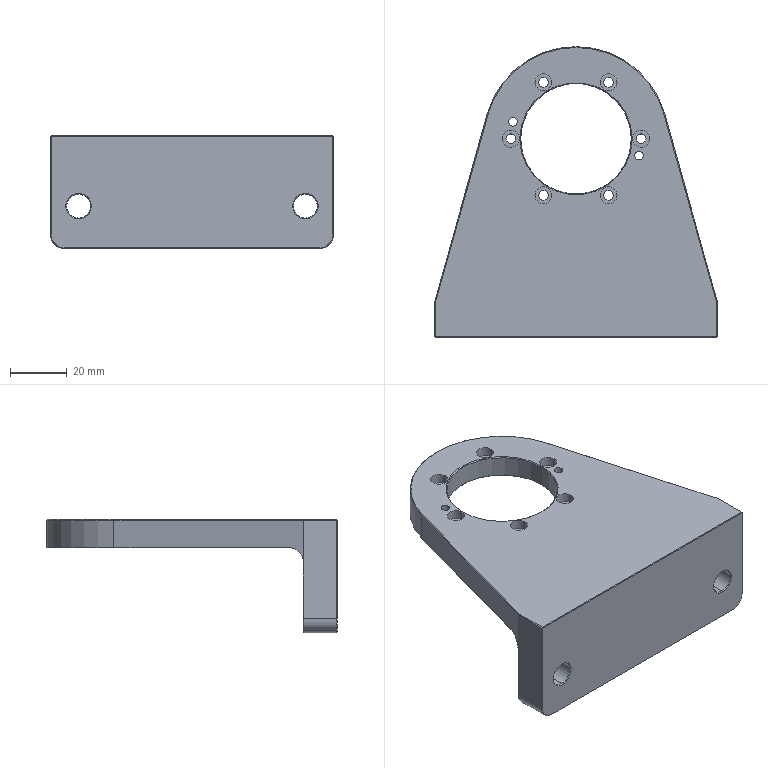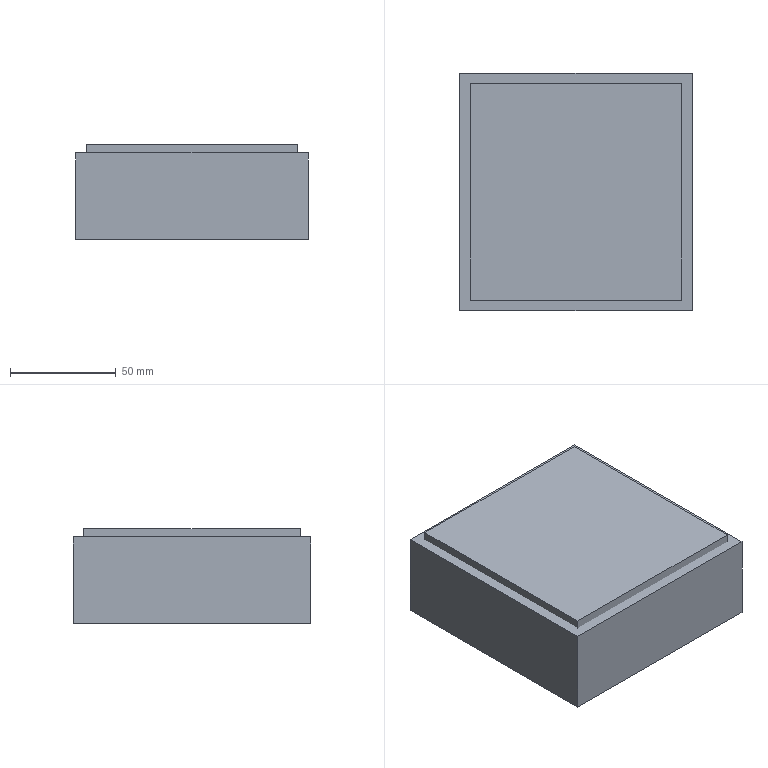CAM job | NX | 3+2 milling, drilling | part box 100 x 102.5 x 40 mm | stock box 110 x 112.5 x 45 mm
Tools:
number,name,description,diameter,corner_radius,flute_length,length,flutes
19,D80,Milling Tool-5 Parameters,80.0,0.0,50.0,75.0,2
1,D6A45,Milling Tool-5 Parameters,6.0,0.0,50.0,75.0,2
16,2.8ZT,Drilling Tool,2.8,0.0,35.0,50.0,2
3,3.4ZT,Drilling Tool,3.4,0.0,35.0,50.0,2
14,D10JING,Milling Tool-5 Parameters,10.0,0.0,50.0,75.0,2
15,D10,Milling Tool-5 Parameters,10.0,0.0,50.0,75.0,2
11,D4,Milling Tool-5 Parameters,4.0,0.0,50.0,75.0,2
17,D2,Milling Tool-5 Parameters,2.0,0.0,50.0,75.0,2
16,D6R0.5,Milling Tool-5 Parameters,6.0,0.5,50.0,75.0,2
20,8.4ZT,Drilling Tool,8.4,0.0,35.0,50.0,2
Operations:
program,operation,operation_type,tool,method,geometry_group,spindle_rpm,surface_speed,feed_per_tooth,feed_cut,feed_plunge,cut_length_mm,path_length_mm,cut_time_min,machine_time_min
1,FLOOR_WALL_COPY,VolumeBased25DMillingOperation,D80,METHOD,A,6500.0,1633.0,0.1154,1500.0,100.0,671.497,725.497,0.4477,0.4531
1,DRILLING_COPY_1,Operation,D6A45,METHOD,A,5000.0,94.0,0.035,350.0,0.0,41.4,308.718,0.1183,0.145
1,DRILLING_COPY_1_COPY,Operation,2.8ZT,METHOD,A,2000.0,17.0,0.0375,150.0,0.0,26.682,162.463,0.1779,0.1915
1,DRILLING_COPY_1_COPY_1,Operation,3.4ZT,METHOD,A,2000.0,21.0,0.045,180.0,0.0,81.129,353.232,0.4507,0.4779
1,ADAPTIVE_MILLING,CavityMilling,D10,METHOD,A,9500.0,298.0,0.1579,3000.0,1000.0,19225.543,19991.279,6.417,6.493
1,HOLE_MILLING,CylinderMilling,D10,METHOD,A,9500.0,0.0,0.0,2200.0,100.0,914.238,983.738,0.4156,0.4225
1,ZLEVEL_PROFILE_COPY_1_COPY_COPY_1,ZLevelMilling,D10JING,METHOD,A,9500.0,298.0,0.0632,1200.0,1000.0,770.852,1010.211,0.6436,0.6675
1,ZLEVEL_PROFILE_COPY_1_COPY_COPY_1_COPY,ZLevelMilling,D10JING,METHOD,A,9500.0,298.0,0.0632,1200.0,1000.0,98.968,176.968,0.0831,0.0909
1,HOLE_MILLING_1,CylinderMilling,D4,METHOD,A,9500.0,119.0,0.0711,1350.0,100.0,477.276,969.676,0.3535,0.4028
1,PLANAR_MILL_COPY_COPY_COPY_COPY_COPY_COPY_1_COPY_1,PlanarMilling,D6A45,METHOD,A,9500.0,179.0,0.0658,1250.0,100.0,609.778,1413.713,0.4878,0.5682
1,刀补17,CylinderMilling,D2,METHOD,A,9500.0,89.0,0.0526,1000.0,100.0,59.436,240.436,0.0594,0.0775
2,ZLEVEL_PROFILE,ZLevelMilling,D10,METHOD,B,9500.0,298.0,0.1053,2000.0,1000.0,2384.552,2437.552,1.216,1.222
2,FLOOR_WALL_COPY_COPY,VolumeBased25DMillingOperation,D80,METHOD,B,6500.0,1633.0,0.1154,1500.0,100.0,3132.485,4193.114,2.088,2.194
2,FLOOR_WALL,VolumeBased25DMillingOperation,D10,METHOD,B,9500.0,298.0,0.1053,2000.0,1000.0,15973.761,16087.461,7.991,8.003
2,ZLEVEL_PROFILE_COPY,ZLevelMilling,D10,METHOD,B,9500.0,298.0,0.1579,3000.0,1000.0,3469.572,3592.997,1.209,1.221
2,HOLE_MILLING_COPY,CylinderMilling,D10JING,METHOD,B,9500.0,298.0,0.0789,1500.0,100.0,483.478,604.978,0.3223,0.3345
2,ZLEVEL_PROFILE_COPY_1_COPY_COPY_1_COPY_1,ZLevelMilling,D10JING,METHOD,B,9500.0,298.0,0.0632,1200.0,1000.0,233.974,442.965,0.1962,0.2171
2,FLOOR_WALL_1,VolumeBased25DMillingOperation,D10JING,METHOD,B,9500.0,298.0,0.0658,1250.0,100.0,1575.069,1913.943,1.26,1.294
2,ZLEVEL_PROFILE_1,ZLevelMilling,D6R0.5,METHOD,B,9500.0,119.0,0.1842,3500.0,100.0,6927.454,7036.504,1.979,1.99
2,ZLEVEL_PROFILE_1_COPY,ZLevelMilling,D6R0.5,METHOD,B,9500.0,119.0,0.1842,3500.0,100.0,2314.901,2538.709,0.6614,0.6838
2,PLANAR_MILL_COPY_COPY_COPY_COPY_COPY_COPY_1_COPY_1_COPY,PlanarMilling,D6A45,METHOD,B,9500.0,179.0,0.0658,1250.0,100.0,233.769,292.769,0.187,0.1929
2,PLANAR_MILL_COPY_COPY_COPY_COPY_COPY_COPY_1_COPY_1_COPY_COPY,PlanarMilling,D6A45,METHOD,B,9500.0,179.0,0.0658,1250.0,100.0,376.944,701.664,0.3016,0.334
2,PLANAR_MILL_COPY_COPY_COPY_COPY_COPY_COPY_1_COPY_1_COPY_COPY_COPY,PlanarMilling,D6A45,METHOD,B,9500.0,179.0,0.0658,1250.0,100.0,124.318,247.318,0.0995,0.1118
3,DRILLING_COPY_1_1,Operation,D6A45,METHOD,C,5000.0,94.0,0.035,350.0,0.0,9.6,162.256,0.0274,0.0427
3,DRILLING_COPY_1_COPY_COPY,Operation,8.4ZT,METHOD,C,2000.0,21.0,0.025,100.0,0.0,38.047,219.151,0.3805,0.3986